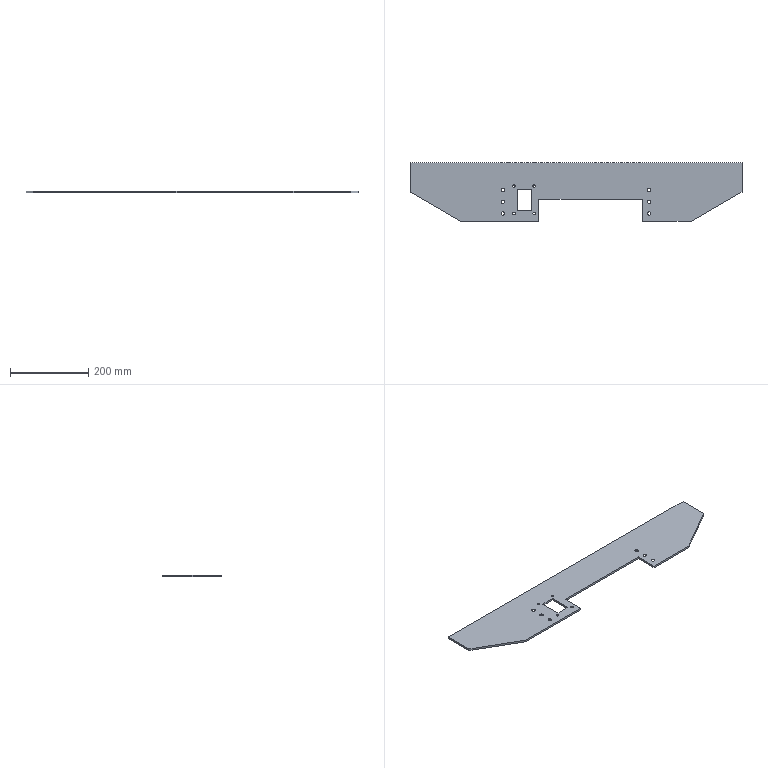Part | NX | features BREP 1 | 1 solid | 36 faces | box 850 x 150 x 5 mm | volume 498141 mm3 | plane 16 | cone 10 | cylinder 10 | commonest cylinder face diameters 9 x6 6.6 x4
STEP:
#1=CARTESIAN_POINT('',(-165.4,90.,-5.));
#2=VERTEX_POINT('',#1);
#3=CARTESIAN_POINT('',(-159.,90.,-5.));
#4=DIRECTION('',(0.,0.,-1.));
#5=DIRECTION('',(-1.,0.,0.));
#6=AXIS2_PLACEMENT_3D('',#3,#4,#5);
#7=CIRCLE('',#6,6.4);
#8=EDGE_CURVE('',#2,#2,#7,.T.);
#9=ORIENTED_EDGE('',*,*,#8,.T.);
#10=EDGE_LOOP('',(#9));
#11=FACE_BOUND('',#10,.T.);
#12=CARTESIAN_POINT('',(-162.3,90.,-1.9));
#13=VERTEX_POINT('',#12);
#14=CARTESIAN_POINT('',(-159.,90.,-1.9));
#15=DIRECTION('',(0.,0.,-1.));
#16=DIRECTION('',(-1.,0.,0.));
#17=AXIS2_PLACEMENT_3D('',#14,#15,#16);
#18=CIRCLE('',#17,3.3);
#19=EDGE_CURVE('',#13,#13,#18,.T.);
#20=ORIENTED_EDGE('',*,*,#19,.F.);
#21=EDGE_LOOP('',(#20));
#22=FACE_BOUND('',#21,.T.);
#23=CARTESIAN_POINT('',(-159.,90.,-5.));
#24=DIRECTION('',(0.,0.,-1.));
#25=DIRECTION('',(-1.,0.,0.));
#26=AXIS2_PLACEMENT_3D('',#23,#24,#25);
#27=CONICAL_SURFACE('',#26,6.4,0.7854);
#28=ADVANCED_FACE('',(#11,#22),#27,.F.);
#29=ORIENTED_EDGE('',*,*,#19,.T.);
#30=EDGE_LOOP('',(#29));
#31=FACE_BOUND('',#30,.T.);
#32=CARTESIAN_POINT('',(-155.7,90.,0.));
#33=VERTEX_POINT('',#32);
#34=CARTESIAN_POINT('',(-159.,90.,0.));
#35=DIRECTION('',(0.,0.,1.));
#36=DIRECTION('',(1.,0.,0.));
#37=AXIS2_PLACEMENT_3D('',#34,#35,#36);
#38=CIRCLE('',#37,3.3);
#39=EDGE_CURVE('',#33,#33,#38,.T.);
#40=ORIENTED_EDGE('',*,*,#39,.T.);
#41=EDGE_LOOP('',(#40));
#42=FACE_BOUND('',#41,.T.);
#43=CARTESIAN_POINT('',(-159.,90.,-5.));
#44=DIRECTION('',(0.,0.,-1.));
#45=DIRECTION('',(-1.,0.,0.));
#46=AXIS2_PLACEMENT_3D('',#43,#44,#45);
#47=CYLINDRICAL_SURFACE('',#46,3.3);
#48=ADVANCED_FACE('',(#31,#42),#47,.F.);
#49=CARTESIAN_POINT('',(-165.4,20.,-5.));
#50=VERTEX_POINT('',#49);
#51=CARTESIAN_POINT('',(-159.,20.,-5.));
#52=DIRECTION('',(0.,0.,-1.));
#53=DIRECTION('',(-1.,0.,0.));
#54=AXIS2_PLACEMENT_3D('',#51,#52,#53);
#55=CIRCLE('',#54,6.4);
#56=EDGE_CURVE('',#50,#50,#55,.T.);
#57=ORIENTED_EDGE('',*,*,#56,.T.);
#58=EDGE_LOOP('',(#57));
#59=FACE_BOUND('',#58,.T.);
#60=CARTESIAN_POINT('',(-162.3,20.,-1.9));
#61=VERTEX_POINT('',#60);
#62=CARTESIAN_POINT('',(-159.,20.,-1.9));
#63=DIRECTION('',(0.,0.,-1.));
#64=DIRECTION('',(-1.,0.,0.));
#65=AXIS2_PLACEMENT_3D('',#62,#63,#64);
#66=CIRCLE('',#65,3.3);
#67=EDGE_CURVE('',#61,#61,#66,.T.);
#68=ORIENTED_EDGE('',*,*,#67,.F.);
#69=EDGE_LOOP('',(#68));
#70=FACE_BOUND('',#69,.T.);
#71=CARTESIAN_POINT('',(-159.,20.,-5.));
#72=DIRECTION('',(0.,0.,-1.));
#73=DIRECTION('',(-1.,0.,0.));
#74=AXIS2_PLACEMENT_3D('',#71,#72,#73);
#75=CONICAL_SURFACE('',#74,6.4,0.7854);
#76=ADVANCED_FACE('',(#59,#70),#75,.F.);
#77=ORIENTED_EDGE('',*,*,#67,.T.);
#78=EDGE_LOOP('',(#77));
#79=FACE_BOUND('',#78,.T.);
#80=CARTESIAN_POINT('',(-155.7,20.,0.));
#81=VERTEX_POINT('',#80);
#82=CARTESIAN_POINT('',(-159.,20.,0.));
#83=DIRECTION('',(0.,0.,1.));
#84=DIRECTION('',(1.,0.,0.));
#85=AXIS2_PLACEMENT_3D('',#82,#83,#84);
#86=CIRCLE('',#85,3.3);
#87=EDGE_CURVE('',#81,#81,#86,.T.);
#88=ORIENTED_EDGE('',*,*,#87,.T.);
#89=EDGE_LOOP('',(#88));
#90=FACE_BOUND('',#89,.T.);
#91=CARTESIAN_POINT('',(-159.,20.,-5.));
#92=DIRECTION('',(0.,0.,-1.));
#93=DIRECTION('',(-1.,0.,0.));
#94=AXIS2_PLACEMENT_3D('',#91,#92,#93);
#95=CYLINDRICAL_SURFACE('',#94,3.3);
#96=ADVANCED_FACE('',(#79,#90),#95,.F.);
#97=CARTESIAN_POINT('',(-113.4,20.,-5.));
#98=VERTEX_POINT('',#97);
#99=CARTESIAN_POINT('',(-107.,20.,-5.));
#100=DIRECTION('',(0.,0.,-1.));
#101=DIRECTION('',(-1.,0.,0.));
#102=AXIS2_PLACEMENT_3D('',#99,#100,#101);
#103=CIRCLE('',#102,6.4);
#104=EDGE_CURVE('',#98,#98,#103,.T.);
#105=ORIENTED_EDGE('',*,*,#104,.T.);
#106=EDGE_LOOP('',(#105));
#107=FACE_BOUND('',#106,.T.);
#108=CARTESIAN_POINT('',(-110.3,20.,-1.9));
#109=VERTEX_POINT('',#108);
#110=CARTESIAN_POINT('',(-107.,20.,-1.9));
#111=DIRECTION('',(0.,0.,-1.));
#112=DIRECTION('',(-1.,0.,0.));
#113=AXIS2_PLACEMENT_3D('',#110,#111,#112);
#114=CIRCLE('',#113,3.3);
#115=EDGE_CURVE('',#109,#109,#114,.T.);
#116=ORIENTED_EDGE('',*,*,#115,.F.);
#117=EDGE_LOOP('',(#116));
#118=FACE_BOUND('',#117,.T.);
#119=CARTESIAN_POINT('',(-107.,20.,-5.));
#120=DIRECTION('',(0.,0.,-1.));
#121=DIRECTION('',(-1.,0.,0.));
#122=AXIS2_PLACEMENT_3D('',#119,#120,#121);
#123=CONICAL_SURFACE('',#122,6.4,0.7854);
#124=ADVANCED_FACE('',(#107,#118),#123,.F.);
#125=ORIENTED_EDGE('',*,*,#115,.T.);
#126=EDGE_LOOP('',(#125));
#127=FACE_BOUND('',#126,.T.);
#128=CARTESIAN_POINT('',(-103.7,20.,0.));
#129=VERTEX_POINT('',#128);
#130=CARTESIAN_POINT('',(-107.,20.,0.));
#131=DIRECTION('',(0.,0.,1.));
#132=DIRECTION('',(1.,0.,0.));
#133=AXIS2_PLACEMENT_3D('',#130,#131,#132);
#134=CIRCLE('',#133,3.3);
#135=EDGE_CURVE('',#129,#129,#134,.T.);
#136=ORIENTED_EDGE('',*,*,#135,.T.);
#137=EDGE_LOOP('',(#136));
#138=FACE_BOUND('',#137,.T.);
#139=CARTESIAN_POINT('',(-107.,20.,-5.));
#140=DIRECTION('',(0.,0.,-1.));
#141=DIRECTION('',(-1.,0.,0.));
#142=AXIS2_PLACEMENT_3D('',#139,#140,#141);
#143=CYLINDRICAL_SURFACE('',#142,3.3);
#144=ADVANCED_FACE('',(#127,#138),#143,.F.);
#145=CARTESIAN_POINT('',(-113.4,90.,-5.));
#146=VERTEX_POINT('',#145);
#147=CARTESIAN_POINT('',(-107.,90.,-5.));
#148=DIRECTION('',(0.,0.,-1.));
#149=DIRECTION('',(-1.,0.,0.));
#150=AXIS2_PLACEMENT_3D('',#147,#148,#149);
#151=CIRCLE('',#150,6.4);
#152=EDGE_CURVE('',#146,#146,#151,.T.);
#153=ORIENTED_EDGE('',*,*,#152,.T.);
#154=EDGE_LOOP('',(#153));
#155=FACE_BOUND('',#154,.T.);
#156=CARTESIAN_POINT('',(-110.3,90.,-1.9));
#157=VERTEX_POINT('',#156);
#158=CARTESIAN_POINT('',(-107.,90.,-1.9));
#159=DIRECTION('',(0.,0.,-1.));
#160=DIRECTION('',(-1.,0.,0.));
#161=AXIS2_PLACEMENT_3D('',#158,#159,#160);
#162=CIRCLE('',#161,3.3);
#163=EDGE_CURVE('',#157,#157,#162,.T.);
#164=ORIENTED_EDGE('',*,*,#163,.F.);
#165=EDGE_LOOP('',(#164));
#166=FACE_BOUND('',#165,.T.);
#167=CARTESIAN_POINT('',(-107.,90.,-5.));
#168=DIRECTION('',(0.,0.,-1.));
#169=DIRECTION('',(-1.,0.,0.));
#170=AXIS2_PLACEMENT_3D('',#167,#168,#169);
#171=CONICAL_SURFACE('',#170,6.4,0.7854);
#172=ADVANCED_FACE('',(#155,#166),#171,.F.);
#173=ORIENTED_EDGE('',*,*,#163,.T.);
#174=EDGE_LOOP('',(#173));
#175=FACE_BOUND('',#174,.T.);
#176=CARTESIAN_POINT('',(-103.7,90.,0.));
#177=VERTEX_POINT('',#176);
#178=CARTESIAN_POINT('',(-107.,90.,0.));
#179=DIRECTION('',(0.,0.,1.));
#180=DIRECTION('',(1.,0.,0.));
#181=AXIS2_PLACEMENT_3D('',#178,#179,#180);
#182=CIRCLE('',#181,3.3);
#183=EDGE_CURVE('',#177,#177,#182,.T.);
#184=ORIENTED_EDGE('',*,*,#183,.T.);
#185=EDGE_LOOP('',(#184));
#186=FACE_BOUND('',#185,.T.);
#187=CARTESIAN_POINT('',(-107.,90.,-5.));
#188=DIRECTION('',(0.,0.,-1.));
#189=DIRECTION('',(-1.,0.,0.));
#190=AXIS2_PLACEMENT_3D('',#187,#188,#189);
#191=CYLINDRICAL_SURFACE('',#190,3.3);
#192=ADVANCED_FACE('',(#175,#186),#191,.F.);
#193=CARTESIAN_POINT('',(-195.8,80.,-5.));
#194=VERTEX_POINT('',#193);
#195=CARTESIAN_POINT('',(-187.,80.,-5.));
#196=DIRECTION('',(0.,0.,-1.));
#197=DIRECTION('',(-1.,0.,0.));
#198=AXIS2_PLACEMENT_3D('',#195,#196,#197);
#199=CIRCLE('',#198,8.8);
#200=EDGE_CURVE('',#194,#194,#199,.T.);
#201=ORIENTED_EDGE('',*,*,#200,.T.);
#202=EDGE_LOOP('',(#201));
#203=FACE_BOUND('',#202,.T.);
#204=CARTESIAN_POINT('',(-191.5,80.,-0.7));
#205=VERTEX_POINT('',#204);
#206=CARTESIAN_POINT('',(-187.,80.,-0.7));
#207=DIRECTION('',(0.,0.,-1.));
#208=DIRECTION('',(-1.,0.,0.));
#209=AXIS2_PLACEMENT_3D('',#206,#207,#208);
#210=CIRCLE('',#209,4.5);
#211=EDGE_CURVE('',#205,#205,#210,.T.);
#212=ORIENTED_EDGE('',*,*,#211,.F.);
#213=EDGE_LOOP('',(#212));
#214=FACE_BOUND('',#213,.T.);
#215=CARTESIAN_POINT('',(-187.,80.,-5.));
#216=DIRECTION('',(0.,0.,-1.));
#217=DIRECTION('',(-1.,0.,0.));
#218=AXIS2_PLACEMENT_3D('',#215,#216,#217);
#219=CONICAL_SURFACE('',#218,8.8,0.7854);
#220=ADVANCED_FACE('',(#203,#214),#219,.F.);
#221=ORIENTED_EDGE('',*,*,#211,.T.);
#222=EDGE_LOOP('',(#221));
#223=FACE_BOUND('',#222,.T.);
#224=CARTESIAN_POINT('',(-191.5,80.,0.));
#225=VERTEX_POINT('',#224);
#226=CARTESIAN_POINT('',(-187.,80.,0.));
#227=DIRECTION('',(0.,0.,-1.));
#228=DIRECTION('',(-1.,0.,0.));
#229=AXIS2_PLACEMENT_3D('',#226,#227,#228);
#230=CIRCLE('',#229,4.5);
#231=EDGE_CURVE('',#225,#225,#230,.T.);
#232=ORIENTED_EDGE('',*,*,#231,.F.);
#233=EDGE_LOOP('',(#232));
#234=FACE_BOUND('',#233,.T.);
#235=CARTESIAN_POINT('',(-187.,80.,-5.));
#236=DIRECTION('',(0.,0.,-1.));
#237=DIRECTION('',(-1.,0.,0.));
#238=AXIS2_PLACEMENT_3D('',#235,#236,#237);
#239=CYLINDRICAL_SURFACE('',#238,4.5);
#240=ADVANCED_FACE('',(#223,#234),#239,.F.);
#241=CARTESIAN_POINT('',(-195.8,50.,-5.));
#242=VERTEX_POINT('',#241);
#243=CARTESIAN_POINT('',(-187.,50.,-5.));
#244=DIRECTION('',(0.,0.,-1.));
#245=DIRECTION('',(-1.,0.,0.));
#246=AXIS2_PLACEMENT_3D('',#243,#244,#245);
#247=CIRCLE('',#246,8.8);
#248=EDGE_CURVE('',#242,#242,#247,.T.);
#249=ORIENTED_EDGE('',*,*,#248,.T.);
#250=EDGE_LOOP('',(#249));
#251=FACE_BOUND('',#250,.T.);
#252=CARTESIAN_POINT('',(-191.5,50.,-0.7));
#253=VERTEX_POINT('',#252);
#254=CARTESIAN_POINT('',(-187.,50.,-0.7));
#255=DIRECTION('',(0.,0.,-1.));
#256=DIRECTION('',(-1.,0.,0.));
#257=AXIS2_PLACEMENT_3D('',#254,#255,#256);
#258=CIRCLE('',#257,4.5);
#259=EDGE_CURVE('',#253,#253,#258,.T.);
#260=ORIENTED_EDGE('',*,*,#259,.F.);
#261=EDGE_LOOP('',(#260));
#262=FACE_BOUND('',#261,.T.);
#263=CARTESIAN_POINT('',(-187.,50.,-5.));
#264=DIRECTION('',(0.,0.,-1.));
#265=DIRECTION('',(-1.,0.,0.));
#266=AXIS2_PLACEMENT_3D('',#263,#264,#265);
#267=CONICAL_SURFACE('',#266,8.8,0.7854);
#268=ADVANCED_FACE('',(#251,#262),#267,.F.);
#269=ORIENTED_EDGE('',*,*,#259,.T.);
#270=EDGE_LOOP('',(#269));
#271=FACE_BOUND('',#270,.T.);
#272=CARTESIAN_POINT('',(-191.5,50.,0.));
#273=VERTEX_POINT('',#272);
#274=CARTESIAN_POINT('',(-187.,50.,0.));
#275=DIRECTION('',(0.,0.,-1.));
#276=DIRECTION('',(-1.,0.,0.));
#277=AXIS2_PLACEMENT_3D('',#274,#275,#276);
#278=CIRCLE('',#277,4.5);
#279=EDGE_CURVE('',#273,#273,#278,.T.);
#280=ORIENTED_EDGE('',*,*,#279,.F.);
#281=EDGE_LOOP('',(#280));
#282=FACE_BOUND('',#281,.T.);
#283=CARTESIAN_POINT('',(-187.,50.,-5.));
#284=DIRECTION('',(0.,0.,-1.));
#285=DIRECTION('',(-1.,0.,0.));
#286=AXIS2_PLACEMENT_3D('',#283,#284,#285);
#287=CYLINDRICAL_SURFACE('',#286,4.5);
#288=ADVANCED_FACE('',(#271,#282),#287,.F.);
#289=CARTESIAN_POINT('',(-195.8,20.,-5.));
#290=VERTEX_POINT('',#289);
#291=CARTESIAN_POINT('',(-187.,20.,-5.));
#292=DIRECTION('',(0.,0.,-1.));
#293=DIRECTION('',(-1.,0.,0.));
#294=AXIS2_PLACEMENT_3D('',#291,#292,#293);
#295=CIRCLE('',#294,8.8);
#296=EDGE_CURVE('',#290,#290,#295,.T.);
#297=ORIENTED_EDGE('',*,*,#296,.T.);
#298=EDGE_LOOP('',(#297));
#299=FACE_BOUND('',#298,.T.);
#300=CARTESIAN_POINT('',(-191.5,20.,-0.7));
#301=VERTEX_POINT('',#300);
#302=CARTESIAN_POINT('',(-187.,20.,-0.7));
#303=DIRECTION('',(0.,0.,-1.));
#304=DIRECTION('',(-1.,0.,0.));
#305=AXIS2_PLACEMENT_3D('',#302,#303,#304);
#306=CIRCLE('',#305,4.5);
#307=EDGE_CURVE('',#301,#301,#306,.T.);
#308=ORIENTED_EDGE('',*,*,#307,.F.);
#309=EDGE_LOOP('',(#308));
#310=FACE_BOUND('',#309,.T.);
#311=CARTESIAN_POINT('',(-187.,20.,-5.));
#312=DIRECTION('',(0.,0.,-1.));
#313=DIRECTION('',(-1.,0.,0.));
#314=AXIS2_PLACEMENT_3D('',#311,#312,#313);
#315=CONICAL_SURFACE('',#314,8.8,0.7854);
#316=ADVANCED_FACE('',(#299,#310),#315,.F.);
#317=ORIENTED_EDGE('',*,*,#307,.T.);
#318=EDGE_LOOP('',(#317));
#319=FACE_BOUND('',#318,.T.);
#320=CARTESIAN_POINT('',(-191.5,20.,0.));
#321=VERTEX_POINT('',#320);
#322=CARTESIAN_POINT('',(-187.,20.,0.));
#323=DIRECTION('',(0.,0.,-1.));
#324=DIRECTION('',(-1.,0.,0.));
#325=AXIS2_PLACEMENT_3D('',#322,#323,#324);
#326=CIRCLE('',#325,4.5);
#327=EDGE_CURVE('',#321,#321,#326,.T.);
#328=ORIENTED_EDGE('',*,*,#327,.F.);
#329=EDGE_LOOP('',(#328));
#330=FACE_BOUND('',#329,.T.);
#331=CARTESIAN_POINT('',(-187.,20.,-5.));
#332=DIRECTION('',(0.,0.,-1.));
#333=DIRECTION('',(-1.,0.,0.));
#334=AXIS2_PLACEMENT_3D('',#331,#332,#333);
#335=CYLINDRICAL_SURFACE('',#334,4.5);
#336=ADVANCED_FACE('',(#319,#330),#335,.F.);
#337=CARTESIAN_POINT('',(178.2,20.,-5.));
#338=VERTEX_POINT('',#337);
#339=CARTESIAN_POINT('',(187.,20.,-5.));
#340=DIRECTION('',(0.,0.,-1.));
#341=DIRECTION('',(-1.,0.,0.));
#342=AXIS2_PLACEMENT_3D('',#339,#340,#341);
#343=CIRCLE('',#342,8.8);
#344=EDGE_CURVE('',#338,#338,#343,.T.);
#345=ORIENTED_EDGE('',*,*,#344,.T.);
#346=EDGE_LOOP('',(#345));
#347=FACE_BOUND('',#346,.T.);
#348=CARTESIAN_POINT('',(182.5,20.,-0.7));
#349=VERTEX_POINT('',#348);
#350=CARTESIAN_POINT('',(187.,20.,-0.7));
#351=DIRECTION('',(0.,0.,-1.));
#352=DIRECTION('',(-1.,0.,0.));
#353=AXIS2_PLACEMENT_3D('',#350,#351,#352);
#354=CIRCLE('',#353,4.5);
#355=EDGE_CURVE('',#349,#349,#354,.T.);
#356=ORIENTED_EDGE('',*,*,#355,.F.);
#357=EDGE_LOOP('',(#356));
#358=FACE_BOUND('',#357,.T.);
#359=CARTESIAN_POINT('',(187.,20.,-5.));
#360=DIRECTION('',(0.,0.,-1.));
#361=DIRECTION('',(-1.,0.,0.));
#362=AXIS2_PLACEMENT_3D('',#359,#360,#361);
#363=CONICAL_SURFACE('',#362,8.8,0.7854);
#364=ADVANCED_FACE('',(#347,#358),#363,.F.);
#365=ORIENTED_EDGE('',*,*,#355,.T.);
#366=EDGE_LOOP('',(#365));
#367=FACE_BOUND('',#366,.T.);
#368=CARTESIAN_POINT('',(182.5,20.,0.));
#369=VERTEX_POINT('',#368);
#370=CARTESIAN_POINT('',(187.,20.,0.));
#371=DIRECTION('',(0.,0.,-1.));
#372=DIRECTION('',(-1.,0.,0.));
#373=AXIS2_PLACEMENT_3D('',#370,#371,#372);
#374=CIRCLE('',#373,4.5);
#375=EDGE_CURVE('',#369,#369,#374,.T.);
#376=ORIENTED_EDGE('',*,*,#375,.F.);
#377=EDGE_LOOP('',(#376));
#378=FACE_BOUND('',#377,.T.);
#379=CARTESIAN_POINT('',(187.,20.,-5.));
#380=DIRECTION('',(0.,0.,-1.));
#381=DIRECTION('',(-1.,0.,0.));
#382=AXIS2_PLACEMENT_3D('',#379,#380,#381);
#383=CYLINDRICAL_SURFACE('',#382,4.5);
#384=ADVANCED_FACE('',(#367,#378),#383,.F.);
#385=CARTESIAN_POINT('',(178.2,50.,-5.));
#386=VERTEX_POINT('',#385);
#387=CARTESIAN_POINT('',(187.,50.,-5.));
#388=DIRECTION('',(0.,0.,-1.));
#389=DIRECTION('',(-1.,0.,0.));
#390=AXIS2_PLACEMENT_3D('',#387,#388,#389);
#391=CIRCLE('',#390,8.8);
#392=EDGE_CURVE('',#386,#386,#391,.T.);
#393=ORIENTED_EDGE('',*,*,#392,.T.);
#394=EDGE_LOOP('',(#393));
#395=FACE_BOUND('',#394,.T.);
#396=CARTESIAN_POINT('',(182.5,50.,-0.7));
#397=VERTEX_POINT('',#396);
#398=CARTESIAN_POINT('',(187.,50.,-0.7));
#399=DIRECTION('',(0.,0.,-1.));
#400=DIRECTION('',(-1.,0.,0.));
#401=AXIS2_PLACEMENT_3D('',#398,#399,#400);
#402=CIRCLE('',#401,4.5);
#403=EDGE_CURVE('',#397,#397,#402,.T.);
#404=ORIENTED_EDGE('',*,*,#403,.F.);
#405=EDGE_LOOP('',(#404));
#406=FACE_BOUND('',#405,.T.);
#407=CARTESIAN_POINT('',(187.,50.,-5.));
#408=DIRECTION('',(0.,0.,-1.));
#409=DIRECTION('',(-1.,0.,0.));
#410=AXIS2_PLACEMENT_3D('',#407,#408,#409);
#411=CONICAL_SURFACE('',#410,8.8,0.7854);
#412=ADVANCED_FACE('',(#395,#406),#411,.F.);
#413=ORIENTED_EDGE('',*,*,#403,.T.);
#414=EDGE_LOOP('',(#413));
#415=FACE_BOUND('',#414,.T.);
#416=CARTESIAN_POINT('',(182.5,50.,0.));
#417=VERTEX_POINT('',#416);
#418=CARTESIAN_POINT('',(187.,50.,0.));
#419=DIRECTION('',(0.,0.,-1.));
#420=DIRECTION('',(-1.,0.,0.));
#421=AXIS2_PLACEMENT_3D('',#418,#419,#420);
#422=CIRCLE('',#421,4.5);
#423=EDGE_CURVE('',#417,#417,#422,.T.);
#424=ORIENTED_EDGE('',*,*,#423,.F.);
#425=EDGE_LOOP('',(#424));
#426=FACE_BOUND('',#425,.T.);
#427=CARTESIAN_POINT('',(187.,50.,-5.));
#428=DIRECTION('',(0.,0.,-1.));
#429=DIRECTION('',(-1.,0.,0.));
#430=AXIS2_PLACEMENT_3D('',#427,#428,#429);
#431=CYLINDRICAL_SURFACE('',#430,4.5);
#432=ADVANCED_FACE('',(#415,#426),#431,.F.);
#433=CARTESIAN_POINT('',(178.2,80.,-5.));
#434=VERTEX_POINT('',#433);
#435=CARTESIAN_POINT('',(187.,80.,-5.));
#436=DIRECTION('',(0.,0.,-1.));
#437=DIRECTION('',(-1.,0.,0.));
#438=AXIS2_PLACEMENT_3D('',#435,#436,#437);
#439=CIRCLE('',#438,8.8);
#440=EDGE_CURVE('',#434,#434,#439,.T.);
#441=ORIENTED_EDGE('',*,*,#440,.T.);
#442=EDGE_LOOP('',(#441));
#443=FACE_BOUND('',#442,.T.);
#444=CARTESIAN_POINT('',(182.5,80.,-0.7));
#445=VERTEX_POINT('',#444);
#446=CARTESIAN_POINT('',(187.,80.,-0.7));
#447=DIRECTION('',(0.,0.,-1.));
#448=DIRECTION('',(-1.,0.,0.));
#449=AXIS2_PLACEMENT_3D('',#446,#447,#448);
#450=CIRCLE('',#449,4.5);
#451=EDGE_CURVE('',#445,#445,#450,.T.);
#452=ORIENTED_EDGE('',*,*,#451,.F.);
#453=EDGE_LOOP('',(#452));
#454=FACE_BOUND('',#453,.T.);
#455=CARTESIAN_POINT('',(187.,80.,-5.));
#456=DIRECTION('',(0.,0.,-1.));
#457=DIRECTION('',(-1.,0.,0.));
#458=AXIS2_PLACEMENT_3D('',#455,#456,#457);
#459=CONICAL_SURFACE('',#458,8.8,0.7854);
#460=ADVANCED_FACE('',(#443,#454),#459,.F.);
#461=ORIENTED_EDGE('',*,*,#451,.T.);
#462=EDGE_LOOP('',(#461));
#463=FACE_BOUND('',#462,.T.);
#464=CARTESIAN_POINT('',(182.5,80.,0.));
#465=VERTEX_POINT('',#464);
#466=CARTESIAN_POINT('',(187.,80.,0.));
#467=DIRECTION('',(0.,0.,-1.));
#468=DIRECTION('',(-1.,0.,0.));
#469=AXIS2_PLACEMENT_3D('',#466,#467,#468);
#470=CIRCLE('',#469,4.5);
#471=EDGE_CURVE('',#465,#465,#470,.T.);
#472=ORIENTED_EDGE('',*,*,#471,.F.);
#473=EDGE_LOOP('',(#472));
#474=FACE_BOUND('',#473,.T.);
#475=CARTESIAN_POINT('',(187.,80.,-5.));
#476=DIRECTION('',(0.,0.,-1.));
#477=DIRECTION('',(-1.,0.,0.));
#478=AXIS2_PLACEMENT_3D('',#475,#476,#477);
#479=CYLINDRICAL_SURFACE('',#478,4.5);
#480=ADVANCED_FACE('',(#463,#474),#479,.F.);
#481=ORIENTED_EDGE('',*,*,#8,.F.);
#482=EDGE_LOOP('',(#481));
#483=FACE_BOUND('',#482,.T.);
#484=ORIENTED_EDGE('',*,*,#56,.F.);
#485=EDGE_LOOP('',(#484));
#486=FACE_BOUND('',#485,.T.);
#487=ORIENTED_EDGE('',*,*,#104,.F.);
#488=EDGE_LOOP('',(#487));
#489=FACE_BOUND('',#488,.T.);
#490=CARTESIAN_POINT('',(-115.,27.,-5.));
#491=VERTEX_POINT('',#490);
#492=CARTESIAN_POINT('',(-151.,27.,-5.));
#493=VERTEX_POINT('',#492);
#494=CARTESIAN_POINT('',(-115.,27.,-5.));
#495=DIRECTION('',(-1.,0.,0.));
#496=VECTOR('',#495,1000.);
#497=LINE('',#494,#496);
#498=EDGE_CURVE('',#491,#493,#497,.T.);
#499=ORIENTED_EDGE('',*,*,#498,.F.);
#500=CARTESIAN_POINT('',(-115.,82.,-5.));
#501=VERTEX_POINT('',#500);
#502=CARTESIAN_POINT('',(-115.,82.,-5.));
#503=DIRECTION('',(0.,-1.,0.));
#504=VECTOR('',#503,1000.);
#505=LINE('',#502,#504);
#506=EDGE_CURVE('',#501,#491,#505,.T.);
#507=ORIENTED_EDGE('',*,*,#506,.F.);
#508=CARTESIAN_POINT('',(-151.,82.,-5.));
#509=VERTEX_POINT('',#508);
#510=CARTESIAN_POINT('',(-115.,82.,-5.));
#511=DIRECTION('',(1.,0.,0.));
#512=VECTOR('',#511,1000.);
#513=LINE('',#510,#512);
#514=EDGE_CURVE('',#509,#501,#513,.T.);
#515=ORIENTED_EDGE('',*,*,#514,.F.);
#516=CARTESIAN_POINT('',(-151.,82.,-5.));
#517=DIRECTION('',(0.,1.,0.));
#518=VECTOR('',#517,1000.);
#519=LINE('',#516,#518);
#520=EDGE_CURVE('',#493,#509,#519,.T.);
#521=ORIENTED_EDGE('',*,*,#520,.F.);
#522=EDGE_LOOP('',(#499,#507,#515,#521));
#523=FACE_BOUND('',#522,.T.);
#524=ORIENTED_EDGE('',*,*,#200,.F.);
#525=EDGE_LOOP('',(#524));
#526=FACE_BOUND('',#525,.T.);
#527=ORIENTED_EDGE('',*,*,#248,.F.);
#528=EDGE_LOOP('',(#527));
#529=FACE_BOUND('',#528,.T.);
#530=ORIENTED_EDGE('',*,*,#296,.F.);
#531=EDGE_LOOP('',(#530));
#532=FACE_BOUND('',#531,.T.);
#533=ORIENTED_EDGE('',*,*,#344,.F.);
#534=EDGE_LOOP('',(#533));
#535=FACE_BOUND('',#534,.T.);
#536=ORIENTED_EDGE('',*,*,#392,.F.);
#537=EDGE_LOOP('',(#536));
#538=FACE_BOUND('',#537,.T.);
#539=ORIENTED_EDGE('',*,*,#440,.F.);
#540=EDGE_LOOP('',(#539));
#541=FACE_BOUND('',#540,.T.);
#542=CARTESIAN_POINT('',(170.,0.,-5.));
#543=VERTEX_POINT('',#542);
#544=CARTESIAN_POINT('',(295.,0.,-5.));
#545=VERTEX_POINT('',#544);
#546=CARTESIAN_POINT('',(-295.,0.,-5.));
#547=DIRECTION('',(1.,0.,0.));
#548=VECTOR('',#547,1000.);
#549=LINE('',#546,#548);
#550=EDGE_CURVE('',#543,#545,#549,.T.);
#551=ORIENTED_EDGE('',*,*,#550,.F.);
#552=CARTESIAN_POINT('',(170.,57.,-5.));
#553=VERTEX_POINT('',#552);
#554=CARTESIAN_POINT('',(170.,57.,-5.));
#555=DIRECTION('',(0.,-1.,0.));
#556=VECTOR('',#555,1000.);
#557=LINE('',#554,#556);
#558=EDGE_CURVE('',#553,#543,#557,.T.);
#559=ORIENTED_EDGE('',*,*,#558,.F.);
#560=CARTESIAN_POINT('',(-95.,57.,-5.));
#561=VERTEX_POINT('',#560);
#562=CARTESIAN_POINT('',(-95.,57.,-5.));
#563=DIRECTION('',(1.,0.,0.));
#564=VECTOR('',#563,1000.);
#565=LINE('',#562,#564);
#566=EDGE_CURVE('',#561,#553,#565,.T.);
#567=ORIENTED_EDGE('',*,*,#566,.F.);
#568=CARTESIAN_POINT('',(-95.,0.,-5.));
#569=VERTEX_POINT('',#568);
#570=CARTESIAN_POINT('',(-95.,57.,-5.));
#571=DIRECTION('',(0.,1.,0.));
#572=VECTOR('',#571,1000.);
#573=LINE('',#570,#572);
#574=EDGE_CURVE('',#569,#561,#573,.T.);
#575=ORIENTED_EDGE('',*,*,#574,.F.);
#576=CARTESIAN_POINT('',(-295.,0.,-5.));
#577=VERTEX_POINT('',#576);
#578=CARTESIAN_POINT('',(-295.,0.,-5.));
#579=DIRECTION('',(1.,0.,0.));
#580=VECTOR('',#579,1000.);
#581=LINE('',#578,#580);
#582=EDGE_CURVE('',#577,#569,#581,.T.);
#583=ORIENTED_EDGE('',*,*,#582,.F.);
#584=CARTESIAN_POINT('',(-425.,75.,-5.));
#585=VERTEX_POINT('',#584);
#586=CARTESIAN_POINT('',(-425.,75.,-5.));
#587=DIRECTION('',(0.8662,-0.4997,0.));
#588=VECTOR('',#587,1000.);
#589=LINE('',#586,#588);
#590=EDGE_CURVE('',#585,#577,#589,.T.);
#591=ORIENTED_EDGE('',*,*,#590,.F.);
#592=CARTESIAN_POINT('',(-425.,150.,-5.));
#593=VERTEX_POINT('',#592);
#594=CARTESIAN_POINT('',(-425.,150.,-5.));
#595=DIRECTION('',(0.,-1.,0.));
#596=VECTOR('',#595,1000.);
#597=LINE('',#594,#596);
#598=EDGE_CURVE('',#593,#585,#597,.T.);
#599=ORIENTED_EDGE('',*,*,#598,.F.);
#600=CARTESIAN_POINT('',(425.,150.,-5.));
#601=VERTEX_POINT('',#600);
#602=CARTESIAN_POINT('',(-425.,150.,-5.));
#603=DIRECTION('',(-1.,0.,0.));
#604=VECTOR('',#603,1000.);
#605=LINE('',#602,#604);
#606=EDGE_CURVE('',#601,#593,#605,.T.);
#607=ORIENTED_EDGE('',*,*,#606,.F.);
#608=CARTESIAN_POINT('',(425.,75.,-5.));
#609=VERTEX_POINT('',#608);
#610=CARTESIAN_POINT('',(425.,150.,-5.));
#611=DIRECTION('',(0.,1.,0.));
#612=VECTOR('',#611,1000.);
#613=LINE('',#610,#612);
#614=EDGE_CURVE('',#609,#601,#613,.T.);
#615=ORIENTED_EDGE('',*,*,#614,.F.);
#616=CARTESIAN_POINT('',(425.,75.,-5.));
#617=DIRECTION('',(0.8662,0.4997,0.));
#618=VECTOR('',#617,1000.);
#619=LINE('',#616,#618);
#620=EDGE_CURVE('',#545,#609,#619,.T.);
#621=ORIENTED_EDGE('',*,*,#620,.F.);
#622=EDGE_LOOP('',(#551,#559,#567,#575,#583,#591,#599,#607,#615,#621));
#623=FACE_BOUND('',#622,.T.);
#624=ORIENTED_EDGE('',*,*,#152,.F.);
#625=EDGE_LOOP('',(#624));
#626=FACE_BOUND('',#625,.T.);
#627=CARTESIAN_POINT('',(0.,0.,-5.));
#628=DIRECTION('',(0.,0.,1.));
#629=DIRECTION('',(1.,0.,0.));
#630=AXIS2_PLACEMENT_3D('',#627,#628,#629);
#631=PLANE('',#630);
#632=ADVANCED_FACE('',(#483,#486,#489,#523,#526,#529,#532,#535,#538,#541,#623,#626),#631,.F.);
#633=CARTESIAN_POINT('',(170.,0.,0.));
#634=VERTEX_POINT('',#633);
#635=CARTESIAN_POINT('',(170.,0.,-5.));
#636=DIRECTION('',(0.,0.,1.));
#637=VECTOR('',#636,1000.);
#638=LINE('',#635,#637);
#639=EDGE_CURVE('',#543,#634,#638,.T.);
#640=ORIENTED_EDGE('',*,*,#639,.F.);
#641=ORIENTED_EDGE('',*,*,#550,.T.);
#642=CARTESIAN_POINT('',(295.,0.,0.));
#643=VERTEX_POINT('',#642);
#644=CARTESIAN_POINT('',(295.,0.,-5.));
#645=DIRECTION('',(0.,0.,1.));
#646=VECTOR('',#645,1000.);
#647=LINE('',#644,#646);
#648=EDGE_CURVE('',#545,#643,#647,.T.);
#649=ORIENTED_EDGE('',*,*,#648,.T.);
#650=CARTESIAN_POINT('',(-295.,0.,0.));
#651=DIRECTION('',(1.,0.,0.));
#652=VECTOR('',#651,1000.);
#653=LINE('',#650,#652);
#654=EDGE_CURVE('',#634,#643,#653,.T.);
#655=ORIENTED_EDGE('',*,*,#654,.F.);
#656=EDGE_LOOP('',(#640,#641,#649,#655));
#657=FACE_BOUND('',#656,.T.);
#658=CARTESIAN_POINT('',(-295.,0.,-5.));
#659=DIRECTION('',(0.,-1.,0.));
#660=DIRECTION('',(1.,0.,0.));
#661=AXIS2_PLACEMENT_3D('',#658,#659,#660);
#662=PLANE('',#661);
#663=ADVANCED_FACE('',(#657),#662,.T.);
#664=CARTESIAN_POINT('',(425.,75.,0.));
#665=VERTEX_POINT('',#664);
#666=CARTESIAN_POINT('',(425.,75.,0.));
#667=DIRECTION('',(0.8662,0.4997,0.));
#668=VECTOR('',#667,1000.);
#669=LINE('',#666,#668);
#670=EDGE_CURVE('',#643,#665,#669,.T.);
#671=ORIENTED_EDGE('',*,*,#670,.F.);
#672=ORIENTED_EDGE('',*,*,#648,.F.);
#673=ORIENTED_EDGE('',*,*,#620,.T.);
#674=CARTESIAN_POINT('',(425.,75.,-5.));
#675=DIRECTION('',(0.,0.,1.));
#676=VECTOR('',#675,1000.);
#677=LINE('',#674,#676);
#678=EDGE_CURVE('',#609,#665,#677,.T.);
#679=ORIENTED_EDGE('',*,*,#678,.T.);
#680=EDGE_LOOP('',(#671,#672,#673,#679));
#681=FACE_BOUND('',#680,.T.);
#682=CARTESIAN_POINT('',(425.,75.,-5.));
#683=DIRECTION('',(0.4997,-0.8662,0.));
#684=DIRECTION('',(0.8662,0.4997,0.));
#685=AXIS2_PLACEMENT_3D('',#682,#683,#684);
#686=PLANE('',#685);
#687=ADVANCED_FACE('',(#681),#686,.T.);
#688=CARTESIAN_POINT('',(-95.,0.,0.));
#689=VERTEX_POINT('',#688);
#690=CARTESIAN_POINT('',(-95.,0.,-5.));
#691=DIRECTION('',(0.,0.,-1.));
#692=VECTOR('',#691,1000.);
#693=LINE('',#690,#692);
#694=EDGE_CURVE('',#689,#569,#693,.T.);
#695=ORIENTED_EDGE('',*,*,#694,.F.);
#696=CARTESIAN_POINT('',(-295.,0.,0.));
#697=VERTEX_POINT('',#696);
#698=CARTESIAN_POINT('',(-295.,0.,0.));
#699=DIRECTION('',(1.,0.,0.));
#700=VECTOR('',#699,1000.);
#701=LINE('',#698,#700);
#702=EDGE_CURVE('',#697,#689,#701,.T.);
#703=ORIENTED_EDGE('',*,*,#702,.F.);
#704=CARTESIAN_POINT('',(-295.,0.,-5.));
#705=DIRECTION('',(0.,0.,1.));
#706=VECTOR('',#705,1000.);
#707=LINE('',#704,#706);
#708=EDGE_CURVE('',#577,#697,#707,.T.);
#709=ORIENTED_EDGE('',*,*,#708,.F.);
#710=ORIENTED_EDGE('',*,*,#582,.T.);
#711=EDGE_LOOP('',(#695,#703,#709,#710));
#712=FACE_BOUND('',#711,.T.);
#713=CARTESIAN_POINT('',(-295.,0.,-5.));
#714=DIRECTION('',(0.,-1.,0.));
#715=DIRECTION('',(1.,0.,0.));
#716=AXIS2_PLACEMENT_3D('',#713,#714,#715);
#717=PLANE('',#716);
#718=ADVANCED_FACE('',(#712),#717,.T.);
#719=CARTESIAN_POINT('',(-425.,75.,0.));
#720=VERTEX_POINT('',#719);
#721=CARTESIAN_POINT('',(-425.,75.,0.));
#722=DIRECTION('',(0.8662,-0.4997,0.));
#723=VECTOR('',#722,1000.);
#724=LINE('',#721,#723);
#725=EDGE_CURVE('',#720,#697,#724,.T.);
#726=ORIENTED_EDGE('',*,*,#725,.F.);
#727=CARTESIAN_POINT('',(-425.,75.,-5.));
#728=DIRECTION('',(0.,0.,1.));
#729=VECTOR('',#728,1000.);
#730=LINE('',#727,#729);
#731=EDGE_CURVE('',#585,#720,#730,.T.);
#732=ORIENTED_EDGE('',*,*,#731,.F.);
#733=ORIENTED_EDGE('',*,*,#590,.T.);
#734=ORIENTED_EDGE('',*,*,#708,.T.);
#735=EDGE_LOOP('',(#726,#732,#733,#734));
#736=FACE_BOUND('',#735,.T.);
#737=CARTESIAN_POINT('',(-425.,75.,-5.));
#738=DIRECTION('',(-0.4997,-0.8662,0.));
#739=DIRECTION('',(0.8662,-0.4997,0.));
#740=AXIS2_PLACEMENT_3D('',#737,#738,#739);
#741=PLANE('',#740);
#742=ADVANCED_FACE('',(#736),#741,.T.);
#743=CARTESIAN_POINT('',(-425.,150.,0.));
#744=VERTEX_POINT('',#743);
#745=CARTESIAN_POINT('',(-425.,150.,0.));
#746=DIRECTION('',(0.,-1.,0.));
#747=VECTOR('',#746,1000.);
#748=LINE('',#745,#747);
#749=EDGE_CURVE('',#744,#720,#748,.T.);
#750=ORIENTED_EDGE('',*,*,#749,.F.);
#751=CARTESIAN_POINT('',(-425.,150.,-5.));
#752=DIRECTION('',(0.,0.,1.));
#753=VECTOR('',#752,1000.);
#754=LINE('',#751,#753);
#755=EDGE_CURVE('',#593,#744,#754,.T.);
#756=ORIENTED_EDGE('',*,*,#755,.F.);
#757=ORIENTED_EDGE('',*,*,#598,.T.);
#758=ORIENTED_EDGE('',*,*,#731,.T.);
#759=EDGE_LOOP('',(#750,#756,#757,#758));
#760=FACE_BOUND('',#759,.T.);
#761=CARTESIAN_POINT('',(-425.,150.,-5.));
#762=DIRECTION('',(-1.,0.,0.));
#763=DIRECTION('',(0.,-1.,0.));
#764=AXIS2_PLACEMENT_3D('',#761,#762,#763);
#765=PLANE('',#764);
#766=ADVANCED_FACE('',(#760),#765,.T.);
#767=CARTESIAN_POINT('',(425.,150.,0.));
#768=VERTEX_POINT('',#767);
#769=CARTESIAN_POINT('',(-425.,150.,0.));
#770=DIRECTION('',(-1.,0.,0.));
#771=VECTOR('',#770,1000.);
#772=LINE('',#769,#771);
#773=EDGE_CURVE('',#768,#744,#772,.T.);
#774=ORIENTED_EDGE('',*,*,#773,.F.);
#775=CARTESIAN_POINT('',(425.,150.,-5.));
#776=DIRECTION('',(0.,0.,1.));
#777=VECTOR('',#776,1000.);
#778=LINE('',#775,#777);
#779=EDGE_CURVE('',#601,#768,#778,.T.);
#780=ORIENTED_EDGE('',*,*,#779,.F.);
#781=ORIENTED_EDGE('',*,*,#606,.T.);
#782=ORIENTED_EDGE('',*,*,#755,.T.);
#783=EDGE_LOOP('',(#774,#780,#781,#782));
#784=FACE_BOUND('',#783,.T.);
#785=CARTESIAN_POINT('',(-425.,150.,-5.));
#786=DIRECTION('',(0.,1.,0.));
#787=DIRECTION('',(-1.,0.,0.));
#788=AXIS2_PLACEMENT_3D('',#785,#786,#787);
#789=PLANE('',#788);
#790=ADVANCED_FACE('',(#784),#789,.T.);
#791=CARTESIAN_POINT('',(425.,150.,0.));
#792=DIRECTION('',(0.,1.,0.));
#793=VECTOR('',#792,1000.);
#794=LINE('',#791,#793);
#795=EDGE_CURVE('',#665,#768,#794,.T.);
#796=ORIENTED_EDGE('',*,*,#795,.F.);
#797=ORIENTED_EDGE('',*,*,#678,.F.);
#798=ORIENTED_EDGE('',*,*,#614,.T.);
#799=ORIENTED_EDGE('',*,*,#779,.T.);
#800=EDGE_LOOP('',(#796,#797,#798,#799));
#801=FACE_BOUND('',#800,.T.);
#802=CARTESIAN_POINT('',(425.,150.,-5.));
#803=DIRECTION('',(1.,0.,0.));
#804=DIRECTION('',(0.,1.,0.));
#805=AXIS2_PLACEMENT_3D('',#802,#803,#804);
#806=PLANE('',#805);
#807=ADVANCED_FACE('',(#801),#806,.T.);
#808=ORIENTED_EDGE('',*,*,#39,.F.);
#809=EDGE_LOOP('',(#808));
#810=FACE_BOUND('',#809,.T.);
#811=ORIENTED_EDGE('',*,*,#87,.F.);
#812=EDGE_LOOP('',(#811));
#813=FACE_BOUND('',#812,.T.);
#814=ORIENTED_EDGE('',*,*,#135,.F.);
#815=EDGE_LOOP('',(#814));
#816=FACE_BOUND('',#815,.T.);
#817=ORIENTED_EDGE('',*,*,#183,.F.);
#818=EDGE_LOOP('',(#817));
#819=FACE_BOUND('',#818,.T.);
#820=CARTESIAN_POINT('',(-115.,27.,0.));
#821=VERTEX_POINT('',#820);
#822=CARTESIAN_POINT('',(-115.,82.,0.));
#823=VERTEX_POINT('',#822);
#824=CARTESIAN_POINT('',(-115.,0.,0.));
#825=DIRECTION('',(0.,1.,0.));
#826=VECTOR('',#825,1000.);
#827=LINE('',#824,#826);
#828=EDGE_CURVE('',#821,#823,#827,.T.);
#829=ORIENTED_EDGE('',*,*,#828,.F.);
#830=CARTESIAN_POINT('',(-151.,27.,0.));
#831=VERTEX_POINT('',#830);
#832=CARTESIAN_POINT('',(0.,27.,0.));
#833=DIRECTION('',(1.,0.,0.));
#834=VECTOR('',#833,1000.);
#835=LINE('',#832,#834);
#836=EDGE_CURVE('',#831,#821,#835,.T.);
#837=ORIENTED_EDGE('',*,*,#836,.F.);
#838=CARTESIAN_POINT('',(-151.,82.,0.));
#839=VERTEX_POINT('',#838);
#840=CARTESIAN_POINT('',(-151.,0.,0.));
#841=DIRECTION('',(0.,-1.,0.));
#842=VECTOR('',#841,1000.);
#843=LINE('',#840,#842);
#844=EDGE_CURVE('',#839,#831,#843,.T.);
#845=ORIENTED_EDGE('',*,*,#844,.F.);
#846=CARTESIAN_POINT('',(0.,82.,0.));
#847=DIRECTION('',(-1.,0.,0.));
#848=VECTOR('',#847,1000.);
#849=LINE('',#846,#848);
#850=EDGE_CURVE('',#823,#839,#849,.T.);
#851=ORIENTED_EDGE('',*,*,#850,.F.);
#852=EDGE_LOOP('',(#829,#837,#845,#851));
#853=FACE_BOUND('',#852,.T.);
#854=ORIENTED_EDGE('',*,*,#231,.T.);
#855=EDGE_LOOP('',(#854));
#856=FACE_BOUND('',#855,.T.);
#857=ORIENTED_EDGE('',*,*,#279,.T.);
#858=EDGE_LOOP('',(#857));
#859=FACE_BOUND('',#858,.T.);
#860=ORIENTED_EDGE('',*,*,#327,.T.);
#861=EDGE_LOOP('',(#860));
#862=FACE_BOUND('',#861,.T.);
#863=ORIENTED_EDGE('',*,*,#375,.T.);
#864=EDGE_LOOP('',(#863));
#865=FACE_BOUND('',#864,.T.);
#866=ORIENTED_EDGE('',*,*,#423,.T.);
#867=EDGE_LOOP('',(#866));
#868=FACE_BOUND('',#867,.T.);
#869=ORIENTED_EDGE('',*,*,#471,.T.);
#870=EDGE_LOOP('',(#869));
#871=FACE_BOUND('',#870,.T.);
#872=CARTESIAN_POINT('',(170.,57.,0.));
#873=VERTEX_POINT('',#872);
#874=CARTESIAN_POINT('',(170.,0.,0.));
#875=DIRECTION('',(0.,1.,0.));
#876=VECTOR('',#875,1000.);
#877=LINE('',#874,#876);
#878=EDGE_CURVE('',#634,#873,#877,.T.);
#879=ORIENTED_EDGE('',*,*,#878,.F.);
#880=ORIENTED_EDGE('',*,*,#654,.T.);
#881=ORIENTED_EDGE('',*,*,#670,.T.);
#882=ORIENTED_EDGE('',*,*,#795,.T.);
#883=ORIENTED_EDGE('',*,*,#773,.T.);
#884=ORIENTED_EDGE('',*,*,#749,.T.);
#885=ORIENTED_EDGE('',*,*,#725,.T.);
#886=ORIENTED_EDGE('',*,*,#702,.T.);
#887=CARTESIAN_POINT('',(-95.,57.,0.));
#888=VERTEX_POINT('',#887);
#889=CARTESIAN_POINT('',(-95.,0.,0.));
#890=DIRECTION('',(0.,-1.,0.));
#891=VECTOR('',#890,1000.);
#892=LINE('',#889,#891);
#893=EDGE_CURVE('',#888,#689,#892,.T.);
#894=ORIENTED_EDGE('',*,*,#893,.F.);
#895=CARTESIAN_POINT('',(0.,57.,0.));
#896=DIRECTION('',(-1.,0.,0.));
#897=VECTOR('',#896,1000.);
#898=LINE('',#895,#897);
#899=EDGE_CURVE('',#873,#888,#898,.T.);
#900=ORIENTED_EDGE('',*,*,#899,.F.);
#901=EDGE_LOOP('',(#879,#880,#881,#882,#883,#884,#885,#886,#894,#900));
#902=FACE_BOUND('',#901,.T.);
#903=CARTESIAN_POINT('',(0.,0.,0.));
#904=DIRECTION('',(0.,0.,1.));
#905=DIRECTION('',(1.,0.,0.));
#906=AXIS2_PLACEMENT_3D('',#903,#904,#905);
#907=PLANE('',#906);
#908=ADVANCED_FACE('',(#810,#813,#816,#819,#853,#856,#859,#862,#865,#868,#871,#902),#907,.T.);
#909=ORIENTED_EDGE('',*,*,#639,.T.);
#910=ORIENTED_EDGE('',*,*,#878,.T.);
#911=CARTESIAN_POINT('',(170.,57.,5.));
#912=DIRECTION('',(0.,0.,-1.));
#913=VECTOR('',#912,1000.);
#914=LINE('',#911,#913);
#915=EDGE_CURVE('',#873,#553,#914,.T.);
#916=ORIENTED_EDGE('',*,*,#915,.T.);
#917=ORIENTED_EDGE('',*,*,#558,.T.);
#918=EDGE_LOOP('',(#909,#910,#916,#917));
#919=FACE_BOUND('',#918,.T.);
#920=CARTESIAN_POINT('',(170.,57.,5.));
#921=DIRECTION('',(1.,0.,0.));
#922=DIRECTION('',(0.,0.,-1.));
#923=AXIS2_PLACEMENT_3D('',#920,#921,#922);
#924=PLANE('',#923);
#925=ADVANCED_FACE('',(#919),#924,.F.);
#926=ORIENTED_EDGE('',*,*,#899,.T.);
#927=CARTESIAN_POINT('',(-95.,57.,5.));
#928=DIRECTION('',(0.,0.,-1.));
#929=VECTOR('',#928,1000.);
#930=LINE('',#927,#929);
#931=EDGE_CURVE('',#888,#561,#930,.T.);
#932=ORIENTED_EDGE('',*,*,#931,.T.);
#933=ORIENTED_EDGE('',*,*,#566,.T.);
#934=ORIENTED_EDGE('',*,*,#915,.F.);
#935=EDGE_LOOP('',(#926,#932,#933,#934));
#936=FACE_BOUND('',#935,.T.);
#937=CARTESIAN_POINT('',(-95.,57.,5.));
#938=DIRECTION('',(0.,1.,0.));
#939=DIRECTION('',(-1.,0.,0.));
#940=AXIS2_PLACEMENT_3D('',#937,#938,#939);
#941=PLANE('',#940);
#942=ADVANCED_FACE('',(#936),#941,.F.);
#943=ORIENTED_EDGE('',*,*,#694,.T.);
#944=ORIENTED_EDGE('',*,*,#574,.T.);
#945=ORIENTED_EDGE('',*,*,#931,.F.);
#946=ORIENTED_EDGE('',*,*,#893,.T.);
#947=EDGE_LOOP('',(#943,#944,#945,#946));
#948=FACE_BOUND('',#947,.T.);
#949=CARTESIAN_POINT('',(-95.,57.,5.));
#950=DIRECTION('',(-1.,0.,0.));
#951=DIRECTION('',(0.,-1.,0.));
#952=AXIS2_PLACEMENT_3D('',#949,#950,#951);
#953=PLANE('',#952);
#954=ADVANCED_FACE('',(#948),#953,.F.);
#955=ORIENTED_EDGE('',*,*,#828,.T.);
#956=CARTESIAN_POINT('',(-115.,82.,5.));
#957=DIRECTION('',(0.,0.,-1.));
#958=VECTOR('',#957,1000.);
#959=LINE('',#956,#958);
#960=EDGE_CURVE('',#823,#501,#959,.T.);
#961=ORIENTED_EDGE('',*,*,#960,.T.);
#962=ORIENTED_EDGE('',*,*,#506,.T.);
#963=CARTESIAN_POINT('',(-115.,27.,5.));
#964=DIRECTION('',(0.,0.,-1.));
#965=VECTOR('',#964,1000.);
#966=LINE('',#963,#965);
#967=EDGE_CURVE('',#821,#491,#966,.T.);
#968=ORIENTED_EDGE('',*,*,#967,.F.);
#969=EDGE_LOOP('',(#955,#961,#962,#968));
#970=FACE_BOUND('',#969,.T.);
#971=CARTESIAN_POINT('',(-115.,82.,5.));
#972=DIRECTION('',(1.,0.,0.));
#973=DIRECTION('',(0.,1.,0.));
#974=AXIS2_PLACEMENT_3D('',#971,#972,#973);
#975=PLANE('',#974);
#976=ADVANCED_FACE('',(#970),#975,.F.);
#977=ORIENTED_EDGE('',*,*,#850,.T.);
#978=CARTESIAN_POINT('',(-151.,82.,5.));
#979=DIRECTION('',(0.,0.,-1.));
#980=VECTOR('',#979,1000.);
#981=LINE('',#978,#980);
#982=EDGE_CURVE('',#839,#509,#981,.T.);
#983=ORIENTED_EDGE('',*,*,#982,.T.);
#984=ORIENTED_EDGE('',*,*,#514,.T.);
#985=ORIENTED_EDGE('',*,*,#960,.F.);
#986=EDGE_LOOP('',(#977,#983,#984,#985));
#987=FACE_BOUND('',#986,.T.);
#988=CARTESIAN_POINT('',(-115.,82.,5.));
#989=DIRECTION('',(0.,1.,0.));
#990=DIRECTION('',(0.,0.,1.));
#991=AXIS2_PLACEMENT_3D('',#988,#989,#990);
#992=PLANE('',#991);
#993=ADVANCED_FACE('',(#987),#992,.F.);
#994=ORIENTED_EDGE('',*,*,#844,.T.);
#995=CARTESIAN_POINT('',(-151.,27.,5.));
#996=DIRECTION('',(0.,0.,-1.));
#997=VECTOR('',#996,1000.);
#998=LINE('',#995,#997);
#999=EDGE_CURVE('',#831,#493,#998,.T.);
#1000=ORIENTED_EDGE('',*,*,#999,.T.);
#1001=ORIENTED_EDGE('',*,*,#520,.T.);
#1002=ORIENTED_EDGE('',*,*,#982,.F.);
#1003=EDGE_LOOP('',(#994,#1000,#1001,#1002));
#1004=FACE_BOUND('',#1003,.T.);
#1005=CARTESIAN_POINT('',(-151.,82.,5.));
#1006=DIRECTION('',(-1.,0.,0.));
#1007=DIRECTION('',(0.,0.,1.));
#1008=AXIS2_PLACEMENT_3D('',#1005,#1006,#1007);
#1009=PLANE('',#1008);
#1010=ADVANCED_FACE('',(#1004),#1009,.F.);
#1011=ORIENTED_EDGE('',*,*,#836,.T.);
#1012=ORIENTED_EDGE('',*,*,#967,.T.);
#1013=ORIENTED_EDGE('',*,*,#498,.T.);
#1014=ORIENTED_EDGE('',*,*,#999,.F.);
#1015=EDGE_LOOP('',(#1011,#1012,#1013,#1014));
#1016=FACE_BOUND('',#1015,.T.);
#1017=CARTESIAN_POINT('',(-115.,27.,5.));
#1018=DIRECTION('',(0.,-1.,0.));
#1019=DIRECTION('',(0.,0.,-1.));
#1020=AXIS2_PLACEMENT_3D('',#1017,#1018,#1019);
#1021=PLANE('',#1020);
#1022=ADVANCED_FACE('',(#1016),#1021,.F.);
#1023=CLOSED_SHELL('',(#28,#48,#76,#96,#124,#144,#172,#192,#220,#240,#268,#288,#316,#336,#364,#384,#412,#432,#460,#480,#632,#663,#687,#718,#742,#766,#790,#807,#908,#925,#942,#954,#976,#993,#1010,#1022));
#1024=MANIFOLD_SOLID_BREP('',#1023);
#1025=(LENGTH_UNIT()NAMED_UNIT(*)SI_UNIT(.MILLI.,.METRE.));
#1026=UNCERTAINTY_MEASURE_WITH_UNIT(LENGTH_MEASURE(0.00001),#1025,'','');
#1027=(NAMED_UNIT(*)PLANE_ANGLE_UNIT()SI_UNIT($,.RADIAN.));
#1028=(NAMED_UNIT(*)SI_UNIT($,.STERADIAN.)SOLID_ANGLE_UNIT());
#1029=(GEOMETRIC_REPRESENTATION_CONTEXT(3)GLOBAL_UNCERTAINTY_ASSIGNED_CONTEXT((#1026))GLOBAL_UNIT_ASSIGNED_CONTEXT((#1025,#1027,#1028))REPRESENTATION_CONTEXT('',''));
#1030=ADVANCED_BREP_SHAPE_REPRESENTATION('',(#1024),#1029);